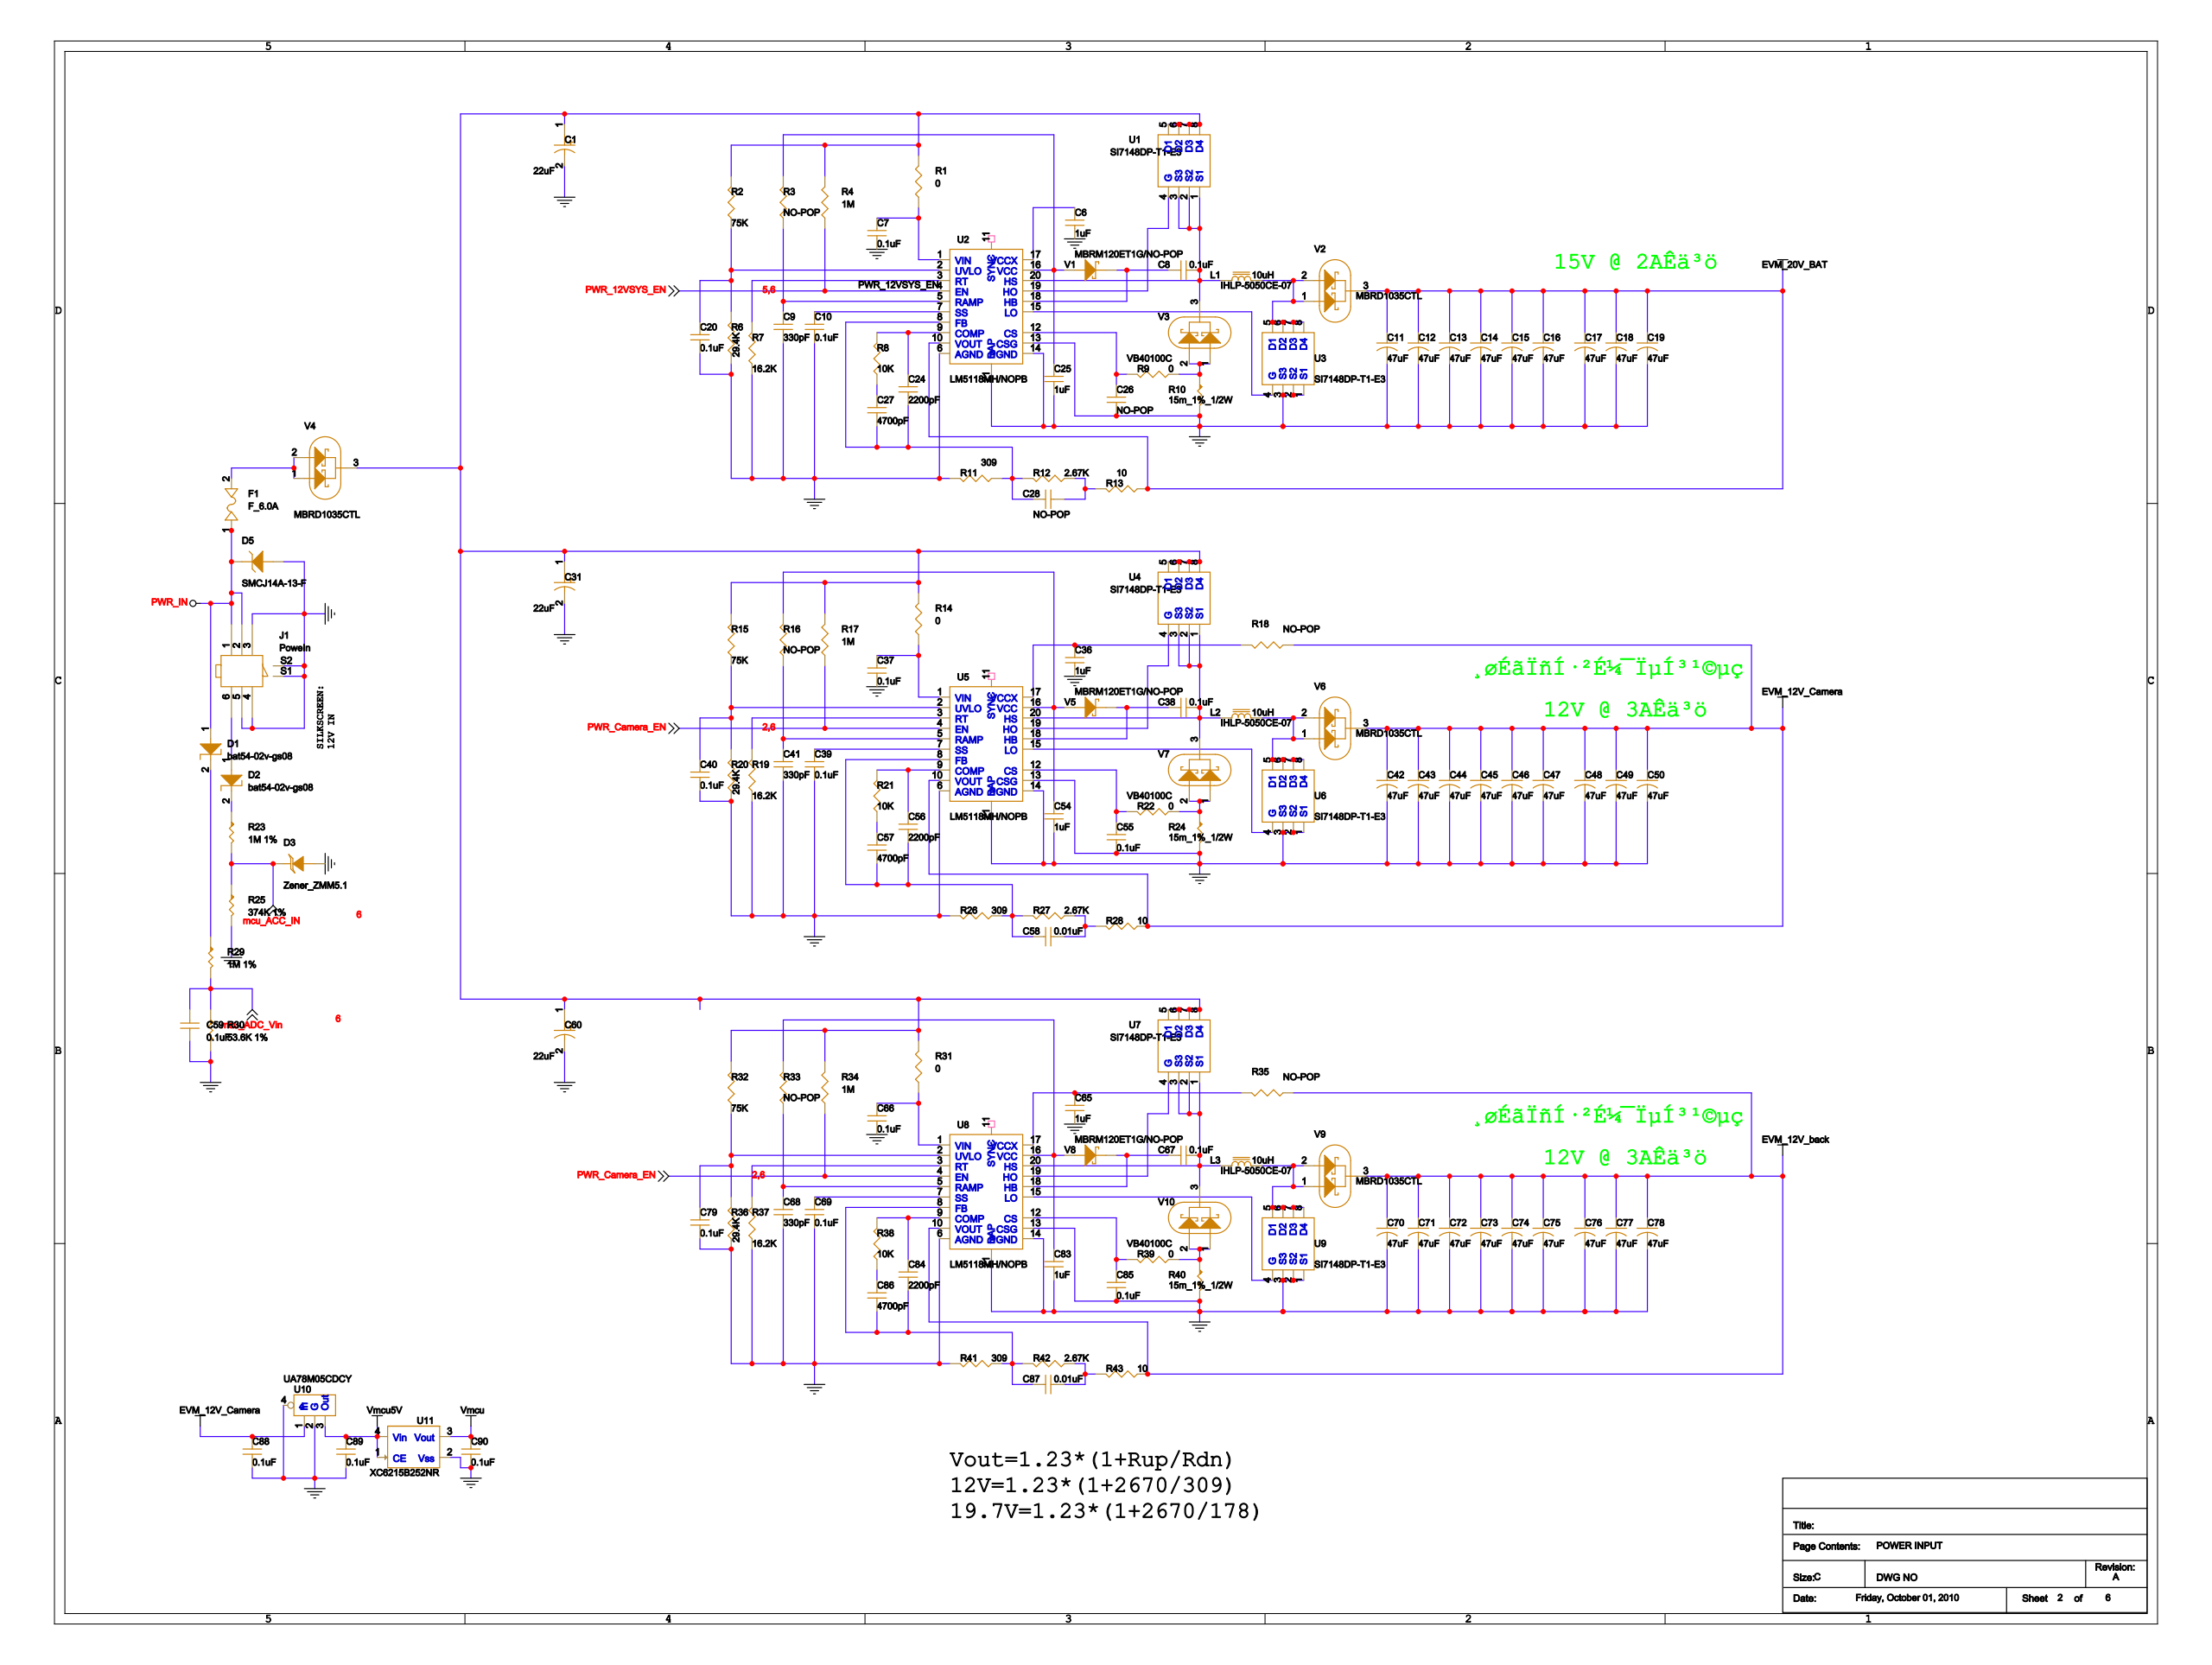Circuit board | Cadence Allegro | 241 parts | 116 nets | one sheet of the schematic
Parts on this sheet (reference | value | footprint):
C6 | 1uF | C0603
C7 | 0.1uF | R0603
C8 | 0.1uF | C0603
C9 | 330pF | C0603
C10 | 0.1uF | C0603
C11 | 47uF | C1210
C12 | 47uF | C1210
C13 | 47uF | C1210
C14 | 47uF | C1210
C15 | 47uF | C1210
C16 | 47uF | C1210
C17 | 47uF | C1210
C18 | 47uF | C1210
C19 | 47uF | C1210
C20 | 0.1uF | C0603
C24 | 2200pF | C0603
C25 | 1uF | C0603
C26 | NO-POP | C0603
C27 | 4700pF | C0603
C28 | NO-POP | C0603
C31 | 22uF | C1210
C36 | 1uF | C0603
C37 | 0.1uF | R0603
C38 | 0.1uF | C0603
C39 | 0.1uF | C0603
C40 | 0.1uF | R0603
C41 | 330pF | C0603
C42 | 47uF | C1210
C43 | 47uF | C1210
C44 | 47uF | C1210
C45 | 47uF | C1210
C46 | 47uF | C1210
C47 | 47uF | C1210
C48 | 47uF | C1210
C49 | 47uF | C1210
C50 | 47uF | C1210
C54 | 1uF | C0603
C55 | 0.1uF | C0603
C56 | 2200pF | C0603
C57 | 4700pF | C0603
C58 | 0.01uF | C0603
C59 | 0.1uF | C0603
C60 | 22uF | C1210
C65 | 1uF | C0603
C66 | 0.1uF | R0603
C67 | 0.1uF | C0603
C68 | 330pF | C0603
C69 | 0.1uF | C0603
C70 | 47uF | C1210
C71 | 47uF | C1210
C72 | 47uF | C1210
C73 | 47uF | C1210
C74 | 47uF | C1210
C75 | 47uF | C1210
C76 | 47uF | C1210
C77 | 47uF | C1210
C78 | 47uF | C1210
C79 | 0.1uF | R0603
C83 | 1uF | C0603
C84 | 2200pF | C0603
C85 | 0.1uF | C0603
C86 | 4700pF | C0603
C87 | 0.01uF | C0603
C88 | 0.1uF | C0603
C89 | 0.1uF | C0603
C90 | 0.1uF | C0603
D1 | bat54-02v-gs08 | SOD_523
D3 | Zener_ZMM5.1 | SOD_123
D5 | SMCJ14A-13-F | DO-214AB
F1 | F_6.0A | FUSEFOLDER-OMNI-BLOK
J1 | PoweIn | HDR4MM2_2X3
L1 | 10uH | L-12X12X7
L2 | 10uH | L-12X12X7
L3 | 10uH | L-12X12X7
R1 | 0 | R0603
R2 | 75K | R0603
R3 | NO-POP | R0603
R4 | 1M | R0603
R7 | 16.2K | R0603
R8 | 10K | R0603
R9 | 0 | R0603
R10 | 15m_1%_1/2W | R1206
R11 | 178 | R0603
R12 | 2.67K | R0603
R13 | 10 | R0603
R14 | 0 | R0603
R15 | 75K | R0603
R16 | NO-POP | R0603
R17 | 1M | R0603
R18 | NO-POP | R0603
R19 | 16.2K | R0603
R21 | 10K | R0603
R22 | 0 | R0603
R23 | 1M 1% | R0603
R24 | 15m_1%_1/2W | R1206
R25 | 374K 1% | R0603
R26 | 309 | R0603
R27 | 2.67K | R0603
R28 | 10 | R0603
R29 | 1M 1% | R0603
R30 | 53.6K 1% | R0603
R31 | 0 | R0603
R32 | 75K | R0603
R33 | NO-POP | R0603
R34 | 1M | R0603
R35 | NO-POP | R0603
R37 | 16.2K | R0603
R38 | 10K | R0603
R39 | 0 | R0603
R40 | 15m_1%_1/2W | R1206
R41 | 309 | R0603
R42 | 2.67K | R0603
R43 | 10 | R0603
U1 | SI7148DP-T1-E3 | SO_8_PAD
U2 | LM5118MH/NOPB | TSSOP-20EP
U3 | SI7148DP-T1-E3 | SO_8_PAD
U4 | SI7148DP-T1-E3 | SO_8_PAD
U5 | LM5118MH/NOPB | TSSOP-20EP
U6 | SI7148DP-T1-E3 | SO_8_PAD
U7 | SI7148DP-T1-E3 | SO_8_PAD
U8 | LM5118MH/NOPB | TSSOP-20EP
U9 | SI7148DP-T1-E3 | SO_8_PAD
U10 | UA78M05CDCY | SOT-223
U11 | XC6215B252NR | SSOT_24
V1 | MBRM120ET1G | DO_216AA
V2 | MBRD1035CTL | TO-252-2
V3 | MBRD1035CTL | TO-263AB
V4 | MBRD1035CTL | TO-252-2
V5 | MBRM120ET1G | DO_216AA
V6 | MBRD1035CTL | TO-252-2
V7 | MBRD1035CTL | TO-263AB
V8 | MBRM120ET1G | DO_216AA
V9 | MBRD1035CTL | TO-252-2
V10 | MBRD1035CTL | TO-263AB
Nets of these parts (net: part-pin ...):
GND: C6-2 C7-2 C9-2 C10-2 C11-2 C12-2 C13-2 C14-2 C15-2 C16-2 C17-2 C18-2 C19-2 C20-2 C25-2 C26-2 C31-2 C36-2 C37-2 C39-2 C40-2 C41-2 C42-2 C43-2 C44-2 C45-2 C46-2 C47-2 C48-2 C49-2 C50-2 C54-2 C55-2 C59-1 C60-2 C65-2 C66-2 C68-2 C69-2 C70-2 C71-2 C72-2 C73-2 C74-2 C75-2 C76-2 C77-2 C78-2 C79-2 C83-2 C85-2 C88-2 C89-2 C90-2 D3-2 D5-2 J1-3 J1-4 J1-5 J1-S1 J1-S2 R7-1 R10-2 R11-2 R19-1 R24-2 R25-2 R26-2 R30-2 R37-1 R40-2 R41-2 U2-6 U2-13 U2-14 U2-21 U3-1 U3-2 U3-3 U5-6 U5-13 U5-14 U5-21 U6-1 U6-2 U6-3 U8-6 U8-13 U8-14 U8-21 U9-1 U9-2 U9-3 U10-2 U10-4 U11-2
N18273157: C31-1 C60-1 R1-2 R2-2 R4-2 R14-2 R15-2 R17-2 R31-2 R32-2 R34-2 U1-5 U1-6 U1-7 U1-8 U4-5 U4-6 U4-7 U4-8 U7-5 U7-6 U7-7 U7-8 V4-3
N18273360: C10-1 U2-7
N18273423: C20-1 R2-1 U2-2
N19220733: C38-1 U5-18 V5-1
N19220705: C38-2 L2-1 U4-1 U4-2 U4-3 U5-20 V7-3
N19220627: C39-1 U5-7
N19220805: C55-1 R22-2 U5-12
MCU_ADC_VIN: C59-2 R29-2 R30-1
N19225166: C67-1 U8-18 V8-1
N19225150: C67-2 L3-1 U7-1 U7-2 U7-3 U8-20 V10-3
N19225070: C69-1 U8-7
N18273505: C8-1 U2-18 V1-1
N18273485: C8-2 L1-1 U1-1 U1-2 U1-3 U2-20 V3-3
N19225248: C85-1 R39-2 U8-12
EVM_12V_CAMERA: C42-1 C43-1 C44-1 C45-1 C46-1 C47-1 C48-1 C49-1 C50-1 C88-1 R18-1 R28-1 U5-10 U10-1 V6-3
VMCU5V: C89-1 U10-3 U11-1 U11-4
VMCU: C90-1 U11-3
N19220558: C37-1 R14-1 U5-1
N19220645: C40-1 R15-1 U5-2
N19224993: C66-1 R31-1 U8-1
N18273233: C7-1 R1-1 U2-1
N19225090: C79-1 R32-1 U8-2
EVM_20V_BAT: C11-1 C12-1 C13-1 C14-1 C15-1 C16-1 C17-1 C18-1 C19-1 R13-1 U2-10 V2-3
EVM_12V_BACK: C70-1 C71-1 C72-1 C73-1 C74-1 C75-1 C76-1 C77-1 C78-1 R35-1 R43-1 U8-10 V9-3
N19220603: C41-1 R16-1 U5-5
N19225029: C68-1 R33-1 U8-5
N18273340: C9-1 R3-1 U2-5
N19220984: C56-2 C57-2 C58-1 R26-1 R27-2 U5-8
N19220439: C58-2 R27-1 R28-2
N19225425: C84-2 C86-2 C87-1 R41-1 R42-2 U8-8
N19224882: C87-2 R42-1 R43-2
N19173758: C27-1 R8-1
N18273840: C24-2 C27-2 C28-1 R11-1 R12-2 U2-8
N19220437: C57-1 R21-1
N19224884: C86-1 R38-1
N18273961: C24-1 R8-2 U2-9
N19221052: C56-1 R21-2 U5-9
N19225489: C84-1 R38-2 U8-9
N18273593: C26-1 R9-2 U2-12
N18273838: C28-2 R12-1 R13-2
PWR_IN: D1-1 D5-1 F1-1 J1-1 J1-2
N18273624: L1-2 U3-5 U3-6 U3-7 U3-8 V2-1 V2-2
N19220840: L2-2 U6-5 U6-6 U6-7 U6-8 V6-1 V6-2
N19225277: L3-2 U9-5 U9-6 U9-7 U9-8 V9-1 V9-2
N19220783: R22-1 R24-1 V7-1 V7-2
N19225218: R39-1 R40-1 V10-1 V10-2
N18273565: R9-1 R10-1 V3-1 V3-2
N19220673: C54-1 R16-2 U5-16 V5-2
N19220473: C36-1 R18-2 U5-17
N18273447: C25-1 R3-2 U2-16 V1-2
N19225118: C83-1 R33-2 U8-16 V8-2
N19224914: C65-1 R35-2 U8-17
PWR_CAMERA_EN: R17-1 R34-1 U5-4 U8-4
PWR_12VSYS_EN: R4-1 U2-4
N19220651: R19-2 U5-3
N19225082: R37-2 U8-3
N18273415: R7-2 U2-3
N19187215: R23-1
MCU_ACC_IN: D3-1 R23-2 R25-1
N18274210: D1-2 R29-1
N18273523: U1-4 U2-19
N18273674: U2-15 U3-4
N18274054: C6-1 U2-17
N19220745: U4-4 U5-19
N19220872: U5-15 U6-4
N19225174: U7-4 U8-19
N19225303: U8-15 U9-4
N19169240: F1-2 V4-1 V4-2
N18273175: J1-6